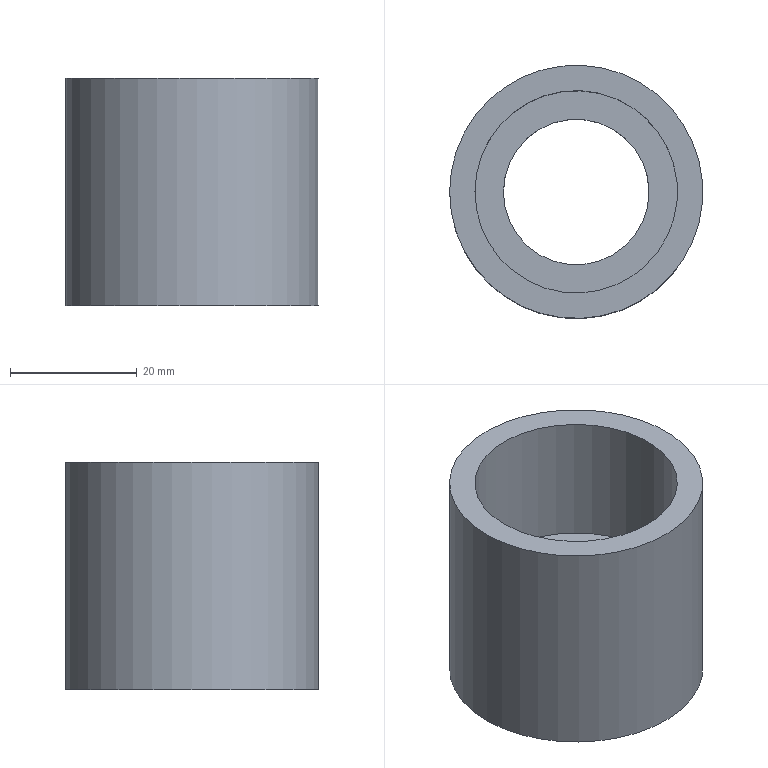Part | NX | features solid 2 | 1 solid | 6 faces | box 40 x 40 x 36 mm | volume 22118 mm3 | cylinder 3 | plane 3 | commonest cylinder face diameters 23 x1 32 x1 40 x1
STEP:
#1=CARTESIAN_POINT('',(105.848,-197.,119.061));
#2=VERTEX_POINT('',#1);
#3=CARTESIAN_POINT('',(121.848,-197.,119.061));
#4=DIRECTION('',(0.,0.,-1.));
#5=DIRECTION('',(-1.,0.,0.));
#6=AXIS2_PLACEMENT_3D('',#3,#4,#5);
#7=CIRCLE('',#6,16.);
#8=EDGE_CURVE('',#2,#2,#7,.T.);
#9=ORIENTED_EDGE('',*,*,#8,.F.);
#10=EDGE_LOOP('',(#9));
#11=FACE_BOUND('',#10,.T.);
#12=CARTESIAN_POINT('',(105.848,-197.,98.061));
#13=VERTEX_POINT('',#12);
#14=CARTESIAN_POINT('',(121.848,-197.,98.061));
#15=DIRECTION('',(0.,0.,-1.));
#16=DIRECTION('',(-1.,0.,0.));
#17=AXIS2_PLACEMENT_3D('',#14,#15,#16);
#18=CIRCLE('',#17,16.);
#19=EDGE_CURVE('',#13,#13,#18,.T.);
#20=ORIENTED_EDGE('',*,*,#19,.T.);
#21=EDGE_LOOP('',(#20));
#22=FACE_BOUND('',#21,.T.);
#23=CARTESIAN_POINT('',(121.848,-197.,93.061));
#24=DIRECTION('',(0.,0.,1.));
#25=DIRECTION('',(-1.,0.,0.));
#26=AXIS2_PLACEMENT_3D('',#23,#24,#25);
#27=CYLINDRICAL_SURFACE('',#26,16.);
#28=ADVANCED_FACE('',(#11,#22),#27,.F.);
#29=CARTESIAN_POINT('',(101.848,-197.,119.061));
#30=VERTEX_POINT('',#29);
#31=CARTESIAN_POINT('',(121.848,-197.,119.061));
#32=DIRECTION('',(0.,0.,-1.));
#33=DIRECTION('',(-1.,0.,0.));
#34=AXIS2_PLACEMENT_3D('',#31,#32,#33);
#35=CIRCLE('',#34,20.);
#36=EDGE_CURVE('',#30,#30,#35,.T.);
#37=ORIENTED_EDGE('',*,*,#36,.F.);
#38=EDGE_LOOP('',(#37));
#39=FACE_BOUND('',#38,.T.);
#40=ORIENTED_EDGE('',*,*,#8,.T.);
#41=EDGE_LOOP('',(#40));
#42=FACE_BOUND('',#41,.T.);
#43=CARTESIAN_POINT('',(121.848,-197.,119.061));
#44=DIRECTION('',(0.,0.,1.));
#45=DIRECTION('',(-1.,0.,0.));
#46=AXIS2_PLACEMENT_3D('',#43,#44,#45);
#47=PLANE('',#46);
#48=ADVANCED_FACE('',(#39,#42),#47,.T.);
#49=CARTESIAN_POINT('',(101.848,-197.,83.061));
#50=VERTEX_POINT('',#49);
#51=CARTESIAN_POINT('',(121.848,-197.,83.061));
#52=DIRECTION('',(0.,0.,-1.));
#53=DIRECTION('',(-1.,0.,0.));
#54=AXIS2_PLACEMENT_3D('',#51,#52,#53);
#55=CIRCLE('',#54,20.);
#56=EDGE_CURVE('',#50,#50,#55,.T.);
#57=ORIENTED_EDGE('',*,*,#56,.T.);
#58=EDGE_LOOP('',(#57));
#59=FACE_BOUND('',#58,.T.);
#60=CARTESIAN_POINT('',(110.348,-197.,83.061));
#61=VERTEX_POINT('',#60);
#62=CARTESIAN_POINT('',(121.848,-197.,83.061));
#63=DIRECTION('',(0.,0.,-1.));
#64=DIRECTION('',(-1.,0.,0.));
#65=AXIS2_PLACEMENT_3D('',#62,#63,#64);
#66=CIRCLE('',#65,11.5);
#67=EDGE_CURVE('',#61,#61,#66,.T.);
#68=ORIENTED_EDGE('',*,*,#67,.F.);
#69=EDGE_LOOP('',(#68));
#70=FACE_BOUND('',#69,.T.);
#71=CARTESIAN_POINT('',(121.848,-197.,83.061));
#72=DIRECTION('',(0.,0.,1.));
#73=DIRECTION('',(-1.,0.,0.));
#74=AXIS2_PLACEMENT_3D('',#71,#72,#73);
#75=PLANE('',#74);
#76=ADVANCED_FACE('',(#59,#70),#75,.F.);
#77=ORIENTED_EDGE('',*,*,#36,.T.);
#78=EDGE_LOOP('',(#77));
#79=FACE_BOUND('',#78,.T.);
#80=ORIENTED_EDGE('',*,*,#56,.F.);
#81=EDGE_LOOP('',(#80));
#82=FACE_BOUND('',#81,.T.);
#83=CARTESIAN_POINT('',(121.848,-197.,93.061));
#84=DIRECTION('',(0.,0.,1.));
#85=DIRECTION('',(-1.,0.,0.));
#86=AXIS2_PLACEMENT_3D('',#83,#84,#85);
#87=CYLINDRICAL_SURFACE('',#86,20.);
#88=ADVANCED_FACE('',(#79,#82),#87,.T.);
#89=CARTESIAN_POINT('',(133.348,-197.,98.061));
#90=VERTEX_POINT('',#89);
#91=CARTESIAN_POINT('',(121.848,-197.,98.061));
#92=DIRECTION('',(0.,0.,1.));
#93=DIRECTION('',(1.,0.,0.));
#94=AXIS2_PLACEMENT_3D('',#91,#92,#93);
#95=CIRCLE('',#94,11.5);
#96=EDGE_CURVE('',#90,#90,#95,.F.);
#97=ORIENTED_EDGE('',*,*,#96,.T.);
#98=EDGE_LOOP('',(#97));
#99=FACE_BOUND('',#98,.T.);
#100=ORIENTED_EDGE('',*,*,#19,.F.);
#101=EDGE_LOOP('',(#100));
#102=FACE_BOUND('',#101,.T.);
#103=CARTESIAN_POINT('',(121.848,-197.,98.061));
#104=DIRECTION('',(0.,0.,-1.));
#105=DIRECTION('',(1.,0.,0.));
#106=AXIS2_PLACEMENT_3D('',#103,#104,#105);
#107=PLANE('',#106);
#108=ADVANCED_FACE('',(#99,#102),#107,.F.);
#109=ORIENTED_EDGE('',*,*,#67,.T.);
#110=EDGE_LOOP('',(#109));
#111=FACE_BOUND('',#110,.T.);
#112=ORIENTED_EDGE('',*,*,#96,.F.);
#113=EDGE_LOOP('',(#112));
#114=FACE_BOUND('',#113,.T.);
#115=CARTESIAN_POINT('',(121.848,-197.,98.061));
#116=DIRECTION('',(0.,0.,-1.));
#117=DIRECTION('',(1.,0.,0.));
#118=AXIS2_PLACEMENT_3D('',#115,#116,#117);
#119=CYLINDRICAL_SURFACE('',#118,11.5);
#120=ADVANCED_FACE('',(#111,#114),#119,.F.);
#121=CLOSED_SHELL('',(#28,#48,#76,#88,#108,#120));
#122=MANIFOLD_SOLID_BREP('',#121);
#123=(LENGTH_UNIT()NAMED_UNIT(*)SI_UNIT(.MILLI.,.METRE.));
#124=UNCERTAINTY_MEASURE_WITH_UNIT(LENGTH_MEASURE(0.00001),#123,'','');
#125=(NAMED_UNIT(*)PLANE_ANGLE_UNIT()SI_UNIT($,.RADIAN.));
#126=(NAMED_UNIT(*)SI_UNIT($,.STERADIAN.)SOLID_ANGLE_UNIT());
#127=(GEOMETRIC_REPRESENTATION_CONTEXT(3)GLOBAL_UNCERTAINTY_ASSIGNED_CONTEXT((#124))GLOBAL_UNIT_ASSIGNED_CONTEXT((#123,#125,#126))REPRESENTATION_CONTEXT('',''));
#128=ADVANCED_BREP_SHAPE_REPRESENTATION('',(#122),#127);